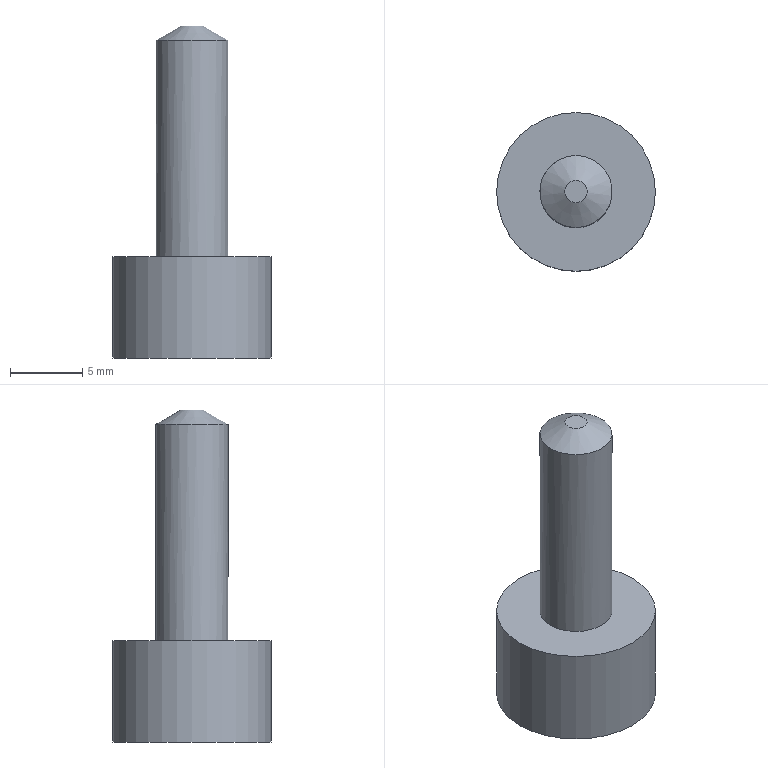Part | STEP file | solid 224 | 1 solid | 6 faces | box 11 x 11 x 23 mm | volume 968.93 mm3 | plane 3 | cylinder 2 | cone 1 | commonest cylinder face diameters 5 x1 11 x1